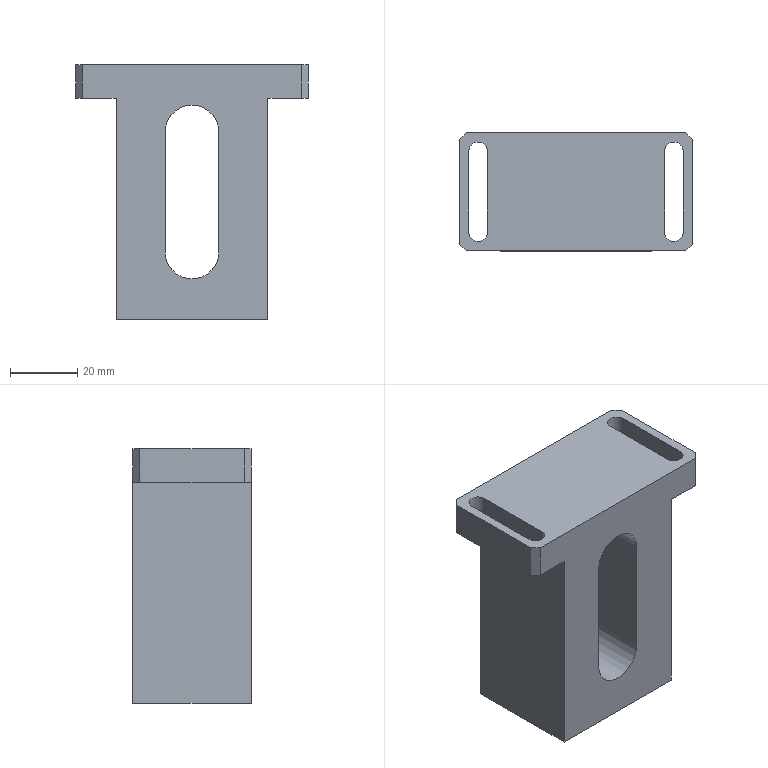Part | STEP file | 11-FG-S01411 | 1 solid | 43 faces | box 69 x 35 x 75.5 mm | volume 96843 mm3 | plane 20 | cylinder 15 | cone 8 | commonest cylinder face diameters 3.3 x8 5.5 x4 16 x3
STEP:
#1=CARTESIAN_POINT('',(23.5,-35.,63.5));
#2=VERTEX_POINT('',#1);
#3=CARTESIAN_POINT('',(31.5,-35.,55.5));
#4=VERTEX_POINT('',#3);
#5=CARTESIAN_POINT('',(23.5,-35.,55.5));
#6=DIRECTION('',(0.,1.,0.));
#7=DIRECTION('',(0.,0.,1.));
#8=AXIS2_PLACEMENT_3D('',#5,#6,#7);
#9=CIRCLE('',#8,8.);
#10=EDGE_CURVE('',#2,#4,#9,.T.);
#11=ORIENTED_EDGE('',*,*,#10,.F.);
#12=CARTESIAN_POINT('',(23.5,0.,63.5));
#13=VERTEX_POINT('',#12);
#14=CARTESIAN_POINT('',(23.5,-40.,63.5));
#15=DIRECTION('',(0.,1.,0.));
#16=VECTOR('',#15,1000.);
#17=LINE('',#14,#16);
#18=EDGE_CURVE('',#2,#13,#17,.T.);
#19=ORIENTED_EDGE('',*,*,#18,.T.);
#20=CARTESIAN_POINT('',(31.5,0.,55.5));
#21=VERTEX_POINT('',#20);
#22=CARTESIAN_POINT('',(23.5,0.,55.5));
#23=DIRECTION('',(0.,1.,0.));
#24=DIRECTION('',(0.,0.,1.));
#25=AXIS2_PLACEMENT_3D('',#22,#23,#24);
#26=CIRCLE('',#25,8.);
#27=EDGE_CURVE('',#13,#21,#26,.T.);
#28=ORIENTED_EDGE('',*,*,#27,.T.);
#29=CARTESIAN_POINT('',(31.5,-40.,55.5));
#30=DIRECTION('',(0.,1.,0.));
#31=VECTOR('',#30,1000.);
#32=LINE('',#29,#31);
#33=EDGE_CURVE('',#4,#21,#32,.T.);
#34=ORIENTED_EDGE('',*,*,#33,.F.);
#35=EDGE_LOOP('',(#11,#19,#28,#34));
#36=FACE_OUTER_BOUND('',#35,.T.);
#37=CARTESIAN_POINT('',(23.5,-40.,55.5));
#38=DIRECTION('',(0.,1.,0.));
#39=DIRECTION('',(0.,0.,1.));
#40=AXIS2_PLACEMENT_3D('',#37,#38,#39);
#41=CYLINDRICAL_SURFACE('',#40,8.);
#42=ADVANCED_FACE('',(#36),#41,.F.);
#43=CARTESIAN_POINT('',(44.15,-7.,10.1));
#44=VERTEX_POINT('',#43);
#45=CARTESIAN_POINT('',(40.85,-7.,10.1));
#46=VERTEX_POINT('',#45);
#47=CARTESIAN_POINT('',(42.5,-7.,10.1));
#48=DIRECTION('',(0.,0.,-1.));
#49=DIRECTION('',(-1.,0.,0.));
#50=AXIS2_PLACEMENT_3D('',#47,#48,#49);
#51=CIRCLE('',#50,1.65);
#52=EDGE_CURVE('',#44,#46,#51,.T.);
#53=ORIENTED_EDGE('',*,*,#52,.F.);
#54=CARTESIAN_POINT('',(44.15,-7.,0.));
#55=VERTEX_POINT('',#54);
#56=CARTESIAN_POINT('',(44.15,-7.,0.));
#57=DIRECTION('',(0.,0.,-1.));
#58=VECTOR('',#57,1000.);
#59=LINE('',#56,#58);
#60=EDGE_CURVE('',#44,#55,#59,.T.);
#61=ORIENTED_EDGE('',*,*,#60,.T.);
#62=CARTESIAN_POINT('',(40.85,-7.,0.));
#63=VERTEX_POINT('',#62);
#64=CARTESIAN_POINT('',(42.5,-7.,0.));
#65=DIRECTION('',(0.,0.,-1.));
#66=DIRECTION('',(-1.,0.,0.));
#67=AXIS2_PLACEMENT_3D('',#64,#65,#66);
#68=CIRCLE('',#67,1.65);
#69=EDGE_CURVE('',#55,#63,#68,.T.);
#70=ORIENTED_EDGE('',*,*,#69,.T.);
#71=CARTESIAN_POINT('',(40.85,-7.,0.));
#72=DIRECTION('',(0.,0.,-1.));
#73=VECTOR('',#72,1000.);
#74=LINE('',#71,#73);
#75=EDGE_CURVE('',#46,#63,#74,.T.);
#76=ORIENTED_EDGE('',*,*,#75,.F.);
#77=EDGE_LOOP('',(#53,#61,#70,#76));
#78=FACE_OUTER_BOUND('',#77,.T.);
#79=CARTESIAN_POINT('',(42.5,-7.,0.));
#80=DIRECTION('',(0.,0.,-1.));
#81=DIRECTION('',(-1.,0.,0.));
#82=AXIS2_PLACEMENT_3D('',#79,#80,#81);
#83=CYLINDRICAL_SURFACE('',#82,1.65);
#84=ADVANCED_FACE('',(#78),#83,.F.);
#85=CARTESIAN_POINT('',(42.5,-7.,11.091));
#86=VERTEX_POINT('',#85);
#87=CARTESIAN_POINT('',(40.85,-7.,10.1));
#88=DIRECTION('',(-0.8572,0.,-0.515));
#89=VECTOR('',#88,1000.);
#90=LINE('',#87,#89);
#91=EDGE_CURVE('',#86,#46,#90,.T.);
#92=ORIENTED_EDGE('',*,*,#91,.F.);
#93=CARTESIAN_POINT('',(44.15,-7.,10.1));
#94=DIRECTION('',(0.8572,0.,-0.515));
#95=VECTOR('',#94,1000.);
#96=LINE('',#93,#95);
#97=EDGE_CURVE('',#86,#44,#96,.T.);
#98=ORIENTED_EDGE('',*,*,#97,.T.);
#99=ORIENTED_EDGE('',*,*,#52,.T.);
#100=EDGE_LOOP('',(#92,#98,#99));
#101=FACE_OUTER_BOUND('',#100,.T.);
#102=CARTESIAN_POINT('',(42.5,-7.,10.1));
#103=DIRECTION('',(0.,0.,-1.));
#104=DIRECTION('',(-1.,0.,0.));
#105=AXIS2_PLACEMENT_3D('',#102,#103,#104);
#106=CONICAL_SURFACE('',#105,1.65,1.03);
#107=ADVANCED_FACE('',(#101),#106,.F.);
#108=CARTESIAN_POINT('',(44.15,-28.,10.1));
#109=VERTEX_POINT('',#108);
#110=CARTESIAN_POINT('',(40.85,-28.,10.1));
#111=VERTEX_POINT('',#110);
#112=CARTESIAN_POINT('',(42.5,-28.,10.1));
#113=DIRECTION('',(0.,0.,-1.));
#114=DIRECTION('',(-1.,0.,0.));
#115=AXIS2_PLACEMENT_3D('',#112,#113,#114);
#116=CIRCLE('',#115,1.65);
#117=EDGE_CURVE('',#109,#111,#116,.T.);
#118=ORIENTED_EDGE('',*,*,#117,.F.);
#119=CARTESIAN_POINT('',(44.15,-28.,0.));
#120=VERTEX_POINT('',#119);
#121=CARTESIAN_POINT('',(44.15,-28.,0.));
#122=DIRECTION('',(0.,0.,-1.));
#123=VECTOR('',#122,1000.);
#124=LINE('',#121,#123);
#125=EDGE_CURVE('',#109,#120,#124,.T.);
#126=ORIENTED_EDGE('',*,*,#125,.T.);
#127=CARTESIAN_POINT('',(40.85,-28.,0.));
#128=VERTEX_POINT('',#127);
#129=CARTESIAN_POINT('',(42.5,-28.,0.));
#130=DIRECTION('',(0.,0.,-1.));
#131=DIRECTION('',(-1.,0.,0.));
#132=AXIS2_PLACEMENT_3D('',#129,#130,#131);
#133=CIRCLE('',#132,1.65);
#134=EDGE_CURVE('',#120,#128,#133,.T.);
#135=ORIENTED_EDGE('',*,*,#134,.T.);
#136=CARTESIAN_POINT('',(40.85,-28.,0.));
#137=DIRECTION('',(0.,0.,-1.));
#138=VECTOR('',#137,1000.);
#139=LINE('',#136,#138);
#140=EDGE_CURVE('',#111,#128,#139,.T.);
#141=ORIENTED_EDGE('',*,*,#140,.F.);
#142=EDGE_LOOP('',(#118,#126,#135,#141));
#143=FACE_OUTER_BOUND('',#142,.T.);
#144=CARTESIAN_POINT('',(42.5,-28.,0.));
#145=DIRECTION('',(0.,0.,-1.));
#146=DIRECTION('',(-1.,0.,0.));
#147=AXIS2_PLACEMENT_3D('',#144,#145,#146);
#148=CYLINDRICAL_SURFACE('',#147,1.65);
#149=ADVANCED_FACE('',(#143),#148,.F.);
#150=CARTESIAN_POINT('',(42.5,-28.,11.091));
#151=VERTEX_POINT('',#150);
#152=CARTESIAN_POINT('',(40.85,-28.,10.1));
#153=DIRECTION('',(-0.8572,0.,-0.515));
#154=VECTOR('',#153,1000.);
#155=LINE('',#152,#154);
#156=EDGE_CURVE('',#151,#111,#155,.T.);
#157=ORIENTED_EDGE('',*,*,#156,.F.);
#158=CARTESIAN_POINT('',(44.15,-28.,10.1));
#159=DIRECTION('',(0.8572,0.,-0.515));
#160=VECTOR('',#159,1000.);
#161=LINE('',#158,#160);
#162=EDGE_CURVE('',#151,#109,#161,.T.);
#163=ORIENTED_EDGE('',*,*,#162,.T.);
#164=ORIENTED_EDGE('',*,*,#117,.T.);
#165=EDGE_LOOP('',(#157,#163,#164));
#166=FACE_OUTER_BOUND('',#165,.T.);
#167=CARTESIAN_POINT('',(42.5,-28.,10.1));
#168=DIRECTION('',(0.,0.,-1.));
#169=DIRECTION('',(-1.,0.,0.));
#170=AXIS2_PLACEMENT_3D('',#167,#168,#169);
#171=CONICAL_SURFACE('',#170,1.65,1.03);
#172=ADVANCED_FACE('',(#166),#171,.F.);
#173=CARTESIAN_POINT('',(6.15,-7.,10.1));
#174=VERTEX_POINT('',#173);
#175=CARTESIAN_POINT('',(2.85,-7.,10.1));
#176=VERTEX_POINT('',#175);
#177=CARTESIAN_POINT('',(4.5,-7.,10.1));
#178=DIRECTION('',(0.,0.,-1.));
#179=DIRECTION('',(-1.,0.,0.));
#180=AXIS2_PLACEMENT_3D('',#177,#178,#179);
#181=CIRCLE('',#180,1.65);
#182=EDGE_CURVE('',#174,#176,#181,.T.);
#183=ORIENTED_EDGE('',*,*,#182,.F.);
#184=CARTESIAN_POINT('',(6.15,-7.,0.));
#185=VERTEX_POINT('',#184);
#186=CARTESIAN_POINT('',(6.15,-7.,0.));
#187=DIRECTION('',(0.,0.,-1.));
#188=VECTOR('',#187,1000.);
#189=LINE('',#186,#188);
#190=EDGE_CURVE('',#174,#185,#189,.T.);
#191=ORIENTED_EDGE('',*,*,#190,.T.);
#192=CARTESIAN_POINT('',(2.85,-7.,0.));
#193=VERTEX_POINT('',#192);
#194=CARTESIAN_POINT('',(4.5,-7.,0.));
#195=DIRECTION('',(0.,0.,-1.));
#196=DIRECTION('',(-1.,0.,0.));
#197=AXIS2_PLACEMENT_3D('',#194,#195,#196);
#198=CIRCLE('',#197,1.65);
#199=EDGE_CURVE('',#185,#193,#198,.T.);
#200=ORIENTED_EDGE('',*,*,#199,.T.);
#201=CARTESIAN_POINT('',(2.85,-7.,0.));
#202=DIRECTION('',(0.,0.,-1.));
#203=VECTOR('',#202,1000.);
#204=LINE('',#201,#203);
#205=EDGE_CURVE('',#176,#193,#204,.T.);
#206=ORIENTED_EDGE('',*,*,#205,.F.);
#207=EDGE_LOOP('',(#183,#191,#200,#206));
#208=FACE_OUTER_BOUND('',#207,.T.);
#209=CARTESIAN_POINT('',(4.5,-7.,0.));
#210=DIRECTION('',(0.,0.,-1.));
#211=DIRECTION('',(-1.,0.,0.));
#212=AXIS2_PLACEMENT_3D('',#209,#210,#211);
#213=CYLINDRICAL_SURFACE('',#212,1.65);
#214=ADVANCED_FACE('',(#208),#213,.F.);
#215=CARTESIAN_POINT('',(4.5,-7.,11.091));
#216=VERTEX_POINT('',#215);
#217=CARTESIAN_POINT('',(2.85,-7.,10.1));
#218=DIRECTION('',(-0.8572,0.,-0.515));
#219=VECTOR('',#218,1000.);
#220=LINE('',#217,#219);
#221=EDGE_CURVE('',#216,#176,#220,.T.);
#222=ORIENTED_EDGE('',*,*,#221,.F.);
#223=CARTESIAN_POINT('',(6.15,-7.,10.1));
#224=DIRECTION('',(0.8572,0.,-0.515));
#225=VECTOR('',#224,1000.);
#226=LINE('',#223,#225);
#227=EDGE_CURVE('',#216,#174,#226,.T.);
#228=ORIENTED_EDGE('',*,*,#227,.T.);
#229=ORIENTED_EDGE('',*,*,#182,.T.);
#230=EDGE_LOOP('',(#222,#228,#229));
#231=FACE_OUTER_BOUND('',#230,.T.);
#232=CARTESIAN_POINT('',(4.5,-7.,10.1));
#233=DIRECTION('',(0.,0.,-1.));
#234=DIRECTION('',(-1.,0.,0.));
#235=AXIS2_PLACEMENT_3D('',#232,#233,#234);
#236=CONICAL_SURFACE('',#235,1.65,1.03);
#237=ADVANCED_FACE('',(#231),#236,.F.);
#238=CARTESIAN_POINT('',(6.15,-28.,10.1));
#239=VERTEX_POINT('',#238);
#240=CARTESIAN_POINT('',(2.85,-28.,10.1));
#241=VERTEX_POINT('',#240);
#242=CARTESIAN_POINT('',(4.5,-28.,10.1));
#243=DIRECTION('',(0.,0.,-1.));
#244=DIRECTION('',(-1.,0.,0.));
#245=AXIS2_PLACEMENT_3D('',#242,#243,#244);
#246=CIRCLE('',#245,1.65);
#247=EDGE_CURVE('',#239,#241,#246,.T.);
#248=ORIENTED_EDGE('',*,*,#247,.F.);
#249=CARTESIAN_POINT('',(6.15,-28.,0.));
#250=VERTEX_POINT('',#249);
#251=CARTESIAN_POINT('',(6.15,-28.,0.));
#252=DIRECTION('',(0.,0.,-1.));
#253=VECTOR('',#252,1000.);
#254=LINE('',#251,#253);
#255=EDGE_CURVE('',#239,#250,#254,.T.);
#256=ORIENTED_EDGE('',*,*,#255,.T.);
#257=CARTESIAN_POINT('',(2.85,-28.,0.));
#258=VERTEX_POINT('',#257);
#259=CARTESIAN_POINT('',(4.5,-28.,0.));
#260=DIRECTION('',(0.,0.,-1.));
#261=DIRECTION('',(-1.,0.,0.));
#262=AXIS2_PLACEMENT_3D('',#259,#260,#261);
#263=CIRCLE('',#262,1.65);
#264=EDGE_CURVE('',#250,#258,#263,.T.);
#265=ORIENTED_EDGE('',*,*,#264,.T.);
#266=CARTESIAN_POINT('',(2.85,-28.,0.));
#267=DIRECTION('',(0.,0.,-1.));
#268=VECTOR('',#267,1000.);
#269=LINE('',#266,#268);
#270=EDGE_CURVE('',#241,#258,#269,.T.);
#271=ORIENTED_EDGE('',*,*,#270,.F.);
#272=EDGE_LOOP('',(#248,#256,#265,#271));
#273=FACE_OUTER_BOUND('',#272,.T.);
#274=CARTESIAN_POINT('',(4.5,-28.,0.));
#275=DIRECTION('',(0.,0.,-1.));
#276=DIRECTION('',(-1.,0.,0.));
#277=AXIS2_PLACEMENT_3D('',#274,#275,#276);
#278=CYLINDRICAL_SURFACE('',#277,1.65);
#279=ADVANCED_FACE('',(#273),#278,.F.);
#280=CARTESIAN_POINT('',(4.5,-28.,11.091));
#281=VERTEX_POINT('',#280);
#282=CARTESIAN_POINT('',(2.85,-28.,10.1));
#283=DIRECTION('',(-0.8572,0.,-0.515));
#284=VECTOR('',#283,1000.);
#285=LINE('',#282,#284);
#286=EDGE_CURVE('',#281,#241,#285,.T.);
#287=ORIENTED_EDGE('',*,*,#286,.F.);
#288=CARTESIAN_POINT('',(6.15,-28.,10.1));
#289=DIRECTION('',(0.8572,0.,-0.515));
#290=VECTOR('',#289,1000.);
#291=LINE('',#288,#290);
#292=EDGE_CURVE('',#281,#239,#291,.T.);
#293=ORIENTED_EDGE('',*,*,#292,.T.);
#294=ORIENTED_EDGE('',*,*,#247,.T.);
#295=EDGE_LOOP('',(#287,#293,#294));
#296=FACE_OUTER_BOUND('',#295,.T.);
#297=CARTESIAN_POINT('',(4.5,-28.,10.1));
#298=DIRECTION('',(0.,0.,-1.));
#299=DIRECTION('',(-1.,0.,0.));
#300=AXIS2_PLACEMENT_3D('',#297,#298,#299);
#301=CONICAL_SURFACE('',#300,1.65,1.03);
#302=ADVANCED_FACE('',(#296),#301,.F.);
#303=CARTESIAN_POINT('',(31.5,-35.,20.));
#304=VERTEX_POINT('',#303);
#305=CARTESIAN_POINT('',(31.5,-35.,75.5));
#306=DIRECTION('',(0.,0.,-1.));
#307=VECTOR('',#306,1000.);
#308=LINE('',#305,#307);
#309=EDGE_CURVE('',#4,#304,#308,.T.);
#310=ORIENTED_EDGE('',*,*,#309,.T.);
#311=CARTESIAN_POINT('',(15.5,-35.,20.));
#312=VERTEX_POINT('',#311);
#313=CARTESIAN_POINT('',(23.5,-35.,20.));
#314=DIRECTION('',(0.,1.,0.));
#315=DIRECTION('',(0.,0.,1.));
#316=AXIS2_PLACEMENT_3D('',#313,#314,#315);
#317=CIRCLE('',#316,8.);
#318=EDGE_CURVE('',#304,#312,#317,.T.);
#319=ORIENTED_EDGE('',*,*,#318,.T.);
#320=CARTESIAN_POINT('',(15.5,-35.,55.5));
#321=VERTEX_POINT('',#320);
#322=CARTESIAN_POINT('',(15.5,-35.,75.5));
#323=DIRECTION('',(0.,0.,1.));
#324=VECTOR('',#323,1000.);
#325=LINE('',#322,#324);
#326=EDGE_CURVE('',#312,#321,#325,.T.);
#327=ORIENTED_EDGE('',*,*,#326,.T.);
#328=CARTESIAN_POINT('',(23.5,-35.,55.5));
#329=DIRECTION('',(0.,1.,0.));
#330=DIRECTION('',(0.,0.,1.));
#331=AXIS2_PLACEMENT_3D('',#328,#329,#330);
#332=CIRCLE('',#331,8.);
#333=EDGE_CURVE('',#321,#2,#332,.T.);
#334=ORIENTED_EDGE('',*,*,#333,.T.);
#335=ORIENTED_EDGE('',*,*,#10,.T.);
#336=EDGE_LOOP('',(#310,#319,#327,#334,#335));
#337=FACE_BOUND('',#336,.T.);
#338=CARTESIAN_POINT('',(-9.,-35.,75.5));
#339=VERTEX_POINT('',#338);
#340=CARTESIAN_POINT('',(56.,-35.,75.5));
#341=VERTEX_POINT('',#340);
#342=CARTESIAN_POINT('',(0.,-35.,75.5));
#343=DIRECTION('',(1.,0.,0.));
#344=VECTOR('',#343,1000.);
#345=LINE('',#342,#344);
#346=EDGE_CURVE('',#339,#341,#345,.T.);
#347=ORIENTED_EDGE('',*,*,#346,.F.);
#348=CARTESIAN_POINT('',(-9.,-35.,65.5));
#349=VERTEX_POINT('',#348);
#350=CARTESIAN_POINT('',(-9.,-35.,65.5));
#351=DIRECTION('',(0.,0.,-1.));
#352=VECTOR('',#351,1000.);
#353=LINE('',#350,#352);
#354=EDGE_CURVE('',#339,#349,#353,.T.);
#355=ORIENTED_EDGE('',*,*,#354,.T.);
#356=CARTESIAN_POINT('',(1.,-35.,65.5));
#357=VERTEX_POINT('',#356);
#358=CARTESIAN_POINT('',(1.,-35.,65.5));
#359=DIRECTION('',(1.,0.,0.));
#360=VECTOR('',#359,1000.);
#361=LINE('',#358,#360);
#362=EDGE_CURVE('',#349,#357,#361,.T.);
#363=ORIENTED_EDGE('',*,*,#362,.T.);
#364=CARTESIAN_POINT('',(1.,-35.,0.));
#365=VERTEX_POINT('',#364);
#366=CARTESIAN_POINT('',(1.,-35.,75.5));
#367=DIRECTION('',(0.,0.,-1.));
#368=VECTOR('',#367,1000.);
#369=LINE('',#366,#368);
#370=EDGE_CURVE('',#357,#365,#369,.T.);
#371=ORIENTED_EDGE('',*,*,#370,.T.);
#372=CARTESIAN_POINT('',(46.,-35.,0.));
#373=VERTEX_POINT('',#372);
#374=CARTESIAN_POINT('',(0.,-35.,0.));
#375=DIRECTION('',(1.,0.,0.));
#376=VECTOR('',#375,1000.);
#377=LINE('',#374,#376);
#378=EDGE_CURVE('',#365,#373,#377,.T.);
#379=ORIENTED_EDGE('',*,*,#378,.T.);
#380=CARTESIAN_POINT('',(46.,-35.,65.5));
#381=VERTEX_POINT('',#380);
#382=CARTESIAN_POINT('',(46.,-35.,75.5));
#383=DIRECTION('',(0.,0.,-1.));
#384=VECTOR('',#383,1000.);
#385=LINE('',#382,#384);
#386=EDGE_CURVE('',#381,#373,#385,.T.);
#387=ORIENTED_EDGE('',*,*,#386,.F.);
#388=CARTESIAN_POINT('',(56.,-35.,65.5));
#389=VERTEX_POINT('',#388);
#390=CARTESIAN_POINT('',(46.,-35.,65.5));
#391=DIRECTION('',(1.,0.,0.));
#392=VECTOR('',#391,1000.);
#393=LINE('',#390,#392);
#394=EDGE_CURVE('',#381,#389,#393,.T.);
#395=ORIENTED_EDGE('',*,*,#394,.T.);
#396=CARTESIAN_POINT('',(56.,-35.,75.5));
#397=DIRECTION('',(0.,0.,1.));
#398=VECTOR('',#397,1000.);
#399=LINE('',#396,#398);
#400=EDGE_CURVE('',#389,#341,#399,.T.);
#401=ORIENTED_EDGE('',*,*,#400,.T.);
#402=EDGE_LOOP('',(#347,#355,#363,#371,#379,#387,#395,#401));
#403=FACE_OUTER_BOUND('',#402,.T.);
#404=CARTESIAN_POINT('',(0.,-35.,75.5));
#405=DIRECTION('',(0.,1.,0.));
#406=DIRECTION('',(0.,0.,1.));
#407=AXIS2_PLACEMENT_3D('',#404,#405,#406);
#408=PLANE('',#407);
#409=ADVANCED_FACE('',(#337,#403),#408,.F.);
#410=CARTESIAN_POINT('',(46.,0.,65.5));
#411=VERTEX_POINT('',#410);
#412=CARTESIAN_POINT('',(46.,0.,0.));
#413=VERTEX_POINT('',#412);
#414=CARTESIAN_POINT('',(46.,0.,75.5));
#415=DIRECTION('',(0.,0.,-1.));
#416=VECTOR('',#415,1000.);
#417=LINE('',#414,#416);
#418=EDGE_CURVE('',#411,#413,#417,.T.);
#419=ORIENTED_EDGE('',*,*,#418,.F.);
#420=CARTESIAN_POINT('',(46.,0.,65.5));
#421=DIRECTION('',(0.,-1.,0.));
#422=VECTOR('',#421,1000.);
#423=LINE('',#420,#422);
#424=EDGE_CURVE('',#411,#381,#423,.T.);
#425=ORIENTED_EDGE('',*,*,#424,.T.);
#426=ORIENTED_EDGE('',*,*,#386,.T.);
#427=CARTESIAN_POINT('',(46.,0.,0.));
#428=DIRECTION('',(0.,1.,0.));
#429=VECTOR('',#428,1000.);
#430=LINE('',#427,#429);
#431=EDGE_CURVE('',#373,#413,#430,.T.);
#432=ORIENTED_EDGE('',*,*,#431,.T.);
#433=EDGE_LOOP('',(#419,#425,#426,#432));
#434=FACE_OUTER_BOUND('',#433,.T.);
#435=CARTESIAN_POINT('',(46.,0.,75.5));
#436=DIRECTION('',(-1.,0.,0.));
#437=DIRECTION('',(0.,0.,1.));
#438=AXIS2_PLACEMENT_3D('',#435,#436,#437);
#439=PLANE('',#438);
#440=ADVANCED_FACE('',(#434),#439,.F.);
#441=CARTESIAN_POINT('',(15.5,0.,20.));
#442=VERTEX_POINT('',#441);
#443=CARTESIAN_POINT('',(15.5,0.,55.5));
#444=VERTEX_POINT('',#443);
#445=CARTESIAN_POINT('',(15.5,0.,20.));
#446=DIRECTION('',(0.,0.,1.));
#447=VECTOR('',#446,1000.);
#448=LINE('',#445,#447);
#449=EDGE_CURVE('',#442,#444,#448,.T.);
#450=ORIENTED_EDGE('',*,*,#449,.F.);
#451=CARTESIAN_POINT('',(31.5,0.,20.));
#452=VERTEX_POINT('',#451);
#453=CARTESIAN_POINT('',(23.5,0.,20.));
#454=DIRECTION('',(0.,1.,0.));
#455=DIRECTION('',(0.,0.,1.));
#456=AXIS2_PLACEMENT_3D('',#453,#454,#455);
#457=CIRCLE('',#456,8.);
#458=EDGE_CURVE('',#452,#442,#457,.T.);
#459=ORIENTED_EDGE('',*,*,#458,.F.);
#460=CARTESIAN_POINT('',(31.5,0.,20.));
#461=DIRECTION('',(0.,0.,-1.));
#462=VECTOR('',#461,1000.);
#463=LINE('',#460,#462);
#464=EDGE_CURVE('',#21,#452,#463,.T.);
#465=ORIENTED_EDGE('',*,*,#464,.F.);
#466=ORIENTED_EDGE('',*,*,#27,.F.);
#467=CARTESIAN_POINT('',(23.5,0.,55.5));
#468=DIRECTION('',(0.,1.,0.));
#469=DIRECTION('',(0.,0.,1.));
#470=AXIS2_PLACEMENT_3D('',#467,#468,#469);
#471=CIRCLE('',#470,8.);
#472=EDGE_CURVE('',#444,#13,#471,.T.);
#473=ORIENTED_EDGE('',*,*,#472,.F.);
#474=EDGE_LOOP('',(#450,#459,#465,#466,#473));
#475=FACE_BOUND('',#474,.T.);
#476=CARTESIAN_POINT('',(1.,0.,65.5));
#477=VERTEX_POINT('',#476);
#478=CARTESIAN_POINT('',(-9.,0.,65.5));
#479=VERTEX_POINT('',#478);
#480=CARTESIAN_POINT('',(1.,0.,65.5));
#481=DIRECTION('',(-1.,0.,0.));
#482=VECTOR('',#481,1000.);
#483=LINE('',#480,#482);
#484=EDGE_CURVE('',#477,#479,#483,.T.);
#485=ORIENTED_EDGE('',*,*,#484,.T.);
#486=CARTESIAN_POINT('',(-9.,0.,75.5));
#487=VERTEX_POINT('',#486);
#488=CARTESIAN_POINT('',(-9.,0.,75.5));
#489=DIRECTION('',(0.,0.,1.));
#490=VECTOR('',#489,1000.);
#491=LINE('',#488,#490);
#492=EDGE_CURVE('',#479,#487,#491,.T.);
#493=ORIENTED_EDGE('',*,*,#492,.T.);
#494=CARTESIAN_POINT('',(56.,0.,75.5));
#495=VERTEX_POINT('',#494);
#496=CARTESIAN_POINT('',(0.,0.,75.5));
#497=DIRECTION('',(-1.,0.,0.));
#498=VECTOR('',#497,1000.);
#499=LINE('',#496,#498);
#500=EDGE_CURVE('',#495,#487,#499,.T.);
#501=ORIENTED_EDGE('',*,*,#500,.F.);
#502=CARTESIAN_POINT('',(56.,0.,65.5));
#503=VERTEX_POINT('',#502);
#504=CARTESIAN_POINT('',(56.,0.,65.5));
#505=DIRECTION('',(0.,0.,-1.));
#506=VECTOR('',#505,1000.);
#507=LINE('',#504,#506);
#508=EDGE_CURVE('',#495,#503,#507,.T.);
#509=ORIENTED_EDGE('',*,*,#508,.T.);
#510=CARTESIAN_POINT('',(46.,0.,65.5));
#511=DIRECTION('',(-1.,0.,0.));
#512=VECTOR('',#511,1000.);
#513=LINE('',#510,#512);
#514=EDGE_CURVE('',#503,#411,#513,.T.);
#515=ORIENTED_EDGE('',*,*,#514,.T.);
#516=ORIENTED_EDGE('',*,*,#418,.T.);
#517=CARTESIAN_POINT('',(1.,0.,0.));
#518=VERTEX_POINT('',#517);
#519=CARTESIAN_POINT('',(0.,0.,0.));
#520=DIRECTION('',(-1.,0.,0.));
#521=VECTOR('',#520,1000.);
#522=LINE('',#519,#521);
#523=EDGE_CURVE('',#413,#518,#522,.T.);
#524=ORIENTED_EDGE('',*,*,#523,.T.);
#525=CARTESIAN_POINT('',(1.,0.,0.));
#526=DIRECTION('',(0.,0.,-1.));
#527=VECTOR('',#526,1000.);
#528=LINE('',#525,#527);
#529=EDGE_CURVE('',#477,#518,#528,.T.);
#530=ORIENTED_EDGE('',*,*,#529,.F.);
#531=EDGE_LOOP('',(#485,#493,#501,#509,#515,#516,#524,#530));
#532=FACE_OUTER_BOUND('',#531,.T.);
#533=CARTESIAN_POINT('',(0.,0.,75.5));
#534=DIRECTION('',(0.,-1.,0.));
#535=DIRECTION('',(0.,0.,-1.));
#536=AXIS2_PLACEMENT_3D('',#533,#534,#535);
#537=PLANE('',#536);
#538=ADVANCED_FACE('',(#475,#532),#537,.F.);
#539=CARTESIAN_POINT('',(-8.25,-5.5,75.5));
#540=VERTEX_POINT('',#539);
#541=CARTESIAN_POINT('',(-2.75,-5.5,75.5));
#542=VERTEX_POINT('',#541);
#543=CARTESIAN_POINT('',(-5.5,-5.5,75.5));
#544=DIRECTION('',(0.,0.,-1.));
#545=DIRECTION('',(-1.,0.,0.));
#546=AXIS2_PLACEMENT_3D('',#543,#544,#545);
#547=CIRCLE('',#546,2.75);
#548=EDGE_CURVE('',#540,#542,#547,.T.);
#549=ORIENTED_EDGE('',*,*,#548,.T.);
#550=CARTESIAN_POINT('',(-2.75,-29.5,75.5));
#551=VERTEX_POINT('',#550);
#552=CARTESIAN_POINT('',(-2.75,-5.5,75.5));
#553=DIRECTION('',(0.,-1.,0.));
#554=VECTOR('',#553,1000.);
#555=LINE('',#552,#554);
#556=EDGE_CURVE('',#542,#551,#555,.T.);
#557=ORIENTED_EDGE('',*,*,#556,.T.);
#558=CARTESIAN_POINT('',(-8.25,-29.5,75.5));
#559=VERTEX_POINT('',#558);
#560=CARTESIAN_POINT('',(-5.5,-29.5,75.5));
#561=DIRECTION('',(0.,0.,-1.));
#562=DIRECTION('',(-1.,0.,0.));
#563=AXIS2_PLACEMENT_3D('',#560,#561,#562);
#564=CIRCLE('',#563,2.75);
#565=EDGE_CURVE('',#551,#559,#564,.T.);
#566=ORIENTED_EDGE('',*,*,#565,.T.);
#567=CARTESIAN_POINT('',(-8.25,-5.5,75.5));
#568=DIRECTION('',(0.,1.,0.));
#569=VECTOR('',#568,1000.);
#570=LINE('',#567,#569);
#571=EDGE_CURVE('',#559,#540,#570,.T.);
#572=ORIENTED_EDGE('',*,*,#571,.T.);
#573=EDGE_LOOP('',(#549,#557,#566,#572));
#574=FACE_BOUND('',#573,.T.);
#575=CARTESIAN_POINT('',(49.75,-5.5,75.5));
#576=VERTEX_POINT('',#575);
#577=CARTESIAN_POINT('',(55.25,-5.5,75.5));
#578=VERTEX_POINT('',#577);
#579=CARTESIAN_POINT('',(52.5,-5.5,75.5));
#580=DIRECTION('',(0.,0.,-1.));
#581=DIRECTION('',(-1.,0.,0.));
#582=AXIS2_PLACEMENT_3D('',#579,#580,#581);
#583=CIRCLE('',#582,2.75);
#584=EDGE_CURVE('',#576,#578,#583,.T.);
#585=ORIENTED_EDGE('',*,*,#584,.T.);
#586=CARTESIAN_POINT('',(55.25,-29.5,75.5));
#587=VERTEX_POINT('',#586);
#588=CARTESIAN_POINT('',(55.25,-5.5,75.5));
#589=DIRECTION('',(0.,-1.,0.));
#590=VECTOR('',#589,1000.);
#591=LINE('',#588,#590);
#592=EDGE_CURVE('',#578,#587,#591,.T.);
#593=ORIENTED_EDGE('',*,*,#592,.T.);
#594=CARTESIAN_POINT('',(49.75,-29.5,75.5));
#595=VERTEX_POINT('',#594);
#596=CARTESIAN_POINT('',(52.5,-29.5,75.5));
#597=DIRECTION('',(0.,0.,-1.));
#598=DIRECTION('',(-1.,0.,0.));
#599=AXIS2_PLACEMENT_3D('',#596,#597,#598);
#600=CIRCLE('',#599,2.75);
#601=EDGE_CURVE('',#587,#595,#600,.T.);
#602=ORIENTED_EDGE('',*,*,#601,.T.);
#603=CARTESIAN_POINT('',(49.75,-5.5,75.5));
#604=DIRECTION('',(0.,1.,0.));
#605=VECTOR('',#604,1000.);
#606=LINE('',#603,#605);
#607=EDGE_CURVE('',#595,#576,#606,.T.);
#608=ORIENTED_EDGE('',*,*,#607,.T.);
#609=EDGE_LOOP('',(#585,#593,#602,#608));
#610=FACE_BOUND('',#609,.T.);
#611=CARTESIAN_POINT('',(-11.,-2.,75.5));
#612=VERTEX_POINT('',#611);
#613=CARTESIAN_POINT('',(-11.,-33.,75.5));
#614=VERTEX_POINT('',#613);
#615=CARTESIAN_POINT('',(-11.,0.,75.5));
#616=DIRECTION('',(0.,-1.,0.));
#617=VECTOR('',#616,1000.);
#618=LINE('',#615,#617);
#619=EDGE_CURVE('',#612,#614,#618,.T.);
#620=ORIENTED_EDGE('',*,*,#619,.T.);
#621=CARTESIAN_POINT('',(-22.,-22.,75.5));
#622=DIRECTION('',(0.7071,-0.7071,0.));
#623=VECTOR('',#622,1000.);
#624=LINE('',#621,#623);
#625=EDGE_CURVE('',#614,#339,#624,.T.);
#626=ORIENTED_EDGE('',*,*,#625,.T.);
#627=ORIENTED_EDGE('',*,*,#346,.T.);
#628=CARTESIAN_POINT('',(58.,-33.,75.5));
#629=VERTEX_POINT('',#628);
#630=CARTESIAN_POINT('',(45.5,-45.5,75.5));
#631=DIRECTION('',(0.7071,0.7071,0.));
#632=VECTOR('',#631,1000.);
#633=LINE('',#630,#632);
#634=EDGE_CURVE('',#341,#629,#633,.T.);
#635=ORIENTED_EDGE('',*,*,#634,.T.);
#636=CARTESIAN_POINT('',(58.,-2.,75.5));
#637=VERTEX_POINT('',#636);
#638=CARTESIAN_POINT('',(58.,0.,75.5));
#639=DIRECTION('',(0.,1.,0.));
#640=VECTOR('',#639,1000.);
#641=LINE('',#638,#640);
#642=EDGE_CURVE('',#629,#637,#641,.T.);
#643=ORIENTED_EDGE('',*,*,#642,.T.);
#644=CARTESIAN_POINT('',(28.,28.,75.5));
#645=DIRECTION('',(-0.7071,0.7071,0.));
#646=VECTOR('',#645,1000.);
#647=LINE('',#644,#646);
#648=EDGE_CURVE('',#637,#495,#647,.T.);
#649=ORIENTED_EDGE('',*,*,#648,.T.);
#650=ORIENTED_EDGE('',*,*,#500,.T.);
#651=CARTESIAN_POINT('',(-4.5,4.5,75.5));
#652=DIRECTION('',(-0.7071,-0.7071,0.));
#653=VECTOR('',#652,1000.);
#654=LINE('',#651,#653);
#655=EDGE_CURVE('',#487,#612,#654,.T.);
#656=ORIENTED_EDGE('',*,*,#655,.T.);
#657=EDGE_LOOP('',(#620,#626,#627,#635,#643,#649,#650,#656));
#658=FACE_OUTER_BOUND('',#657,.T.);
#659=CARTESIAN_POINT('',(0.,0.,75.5));
#660=DIRECTION('',(0.,0.,1.));
#661=DIRECTION('',(1.,0.,0.));
#662=AXIS2_PLACEMENT_3D('',#659,#660,#661);
#663=PLANE('',#662);
#664=ADVANCED_FACE('',(#574,#610,#658),#663,.T.);
#665=CARTESIAN_POINT('',(42.5,-7.,0.));
#666=DIRECTION('',(0.,0.,-1.));
#667=DIRECTION('',(-1.,0.,0.));
#668=AXIS2_PLACEMENT_3D('',#665,#666,#667);
#669=CIRCLE('',#668,1.65);
#670=EDGE_CURVE('',#63,#55,#669,.T.);
#671=ORIENTED_EDGE('',*,*,#670,.F.);
#672=ORIENTED_EDGE('',*,*,#69,.F.);
#673=EDGE_LOOP('',(#671,#672));
#674=FACE_BOUND('',#673,.T.);
#675=CARTESIAN_POINT('',(42.5,-28.,0.));
#676=DIRECTION('',(0.,0.,-1.));
#677=DIRECTION('',(-1.,0.,0.));
#678=AXIS2_PLACEMENT_3D('',#675,#676,#677);
#679=CIRCLE('',#678,1.65);
#680=EDGE_CURVE('',#128,#120,#679,.T.);
#681=ORIENTED_EDGE('',*,*,#680,.F.);
#682=ORIENTED_EDGE('',*,*,#134,.F.);
#683=EDGE_LOOP('',(#681,#682));
#684=FACE_BOUND('',#683,.T.);
#685=CARTESIAN_POINT('',(4.5,-7.,0.));
#686=DIRECTION('',(0.,0.,-1.));
#687=DIRECTION('',(-1.,0.,0.));
#688=AXIS2_PLACEMENT_3D('',#685,#686,#687);
#689=CIRCLE('',#688,1.65);
#690=EDGE_CURVE('',#193,#185,#689,.T.);
#691=ORIENTED_EDGE('',*,*,#690,.F.);
#692=ORIENTED_EDGE('',*,*,#199,.F.);
#693=EDGE_LOOP('',(#691,#692));
#694=FACE_BOUND('',#693,.T.);
#695=CARTESIAN_POINT('',(4.5,-28.,0.));
#696=DIRECTION('',(0.,0.,-1.));
#697=DIRECTION('',(-1.,0.,0.));
#698=AXIS2_PLACEMENT_3D('',#695,#696,#697);
#699=CIRCLE('',#698,1.65);
#700=EDGE_CURVE('',#258,#250,#699,.T.);
#701=ORIENTED_EDGE('',*,*,#700,.F.);
#702=ORIENTED_EDGE('',*,*,#264,.F.);
#703=EDGE_LOOP('',(#701,#702));
#704=FACE_BOUND('',#703,.T.);
#705=ORIENTED_EDGE('',*,*,#378,.F.);
#706=CARTESIAN_POINT('',(1.,0.,0.));
#707=DIRECTION('',(0.,1.,0.));
#708=VECTOR('',#707,1000.);
#709=LINE('',#706,#708);
#710=EDGE_CURVE('',#365,#518,#709,.T.);
#711=ORIENTED_EDGE('',*,*,#710,.T.);
#712=ORIENTED_EDGE('',*,*,#523,.F.);
#713=ORIENTED_EDGE('',*,*,#431,.F.);
#714=EDGE_LOOP('',(#705,#711,#712,#713));
#715=FACE_OUTER_BOUND('',#714,.T.);
#716=CARTESIAN_POINT('',(0.,0.,0.));
#717=DIRECTION('',(0.,0.,1.));
#718=DIRECTION('',(1.,0.,0.));
#719=AXIS2_PLACEMENT_3D('',#716,#717,#718);
#720=PLANE('',#719);
#721=ADVANCED_FACE('',(#674,#684,#694,#704,#715),#720,.F.);
#722=ORIENTED_EDGE('',*,*,#370,.F.);
#723=CARTESIAN_POINT('',(1.,0.,65.5));
#724=DIRECTION('',(0.,1.,0.));
#725=VECTOR('',#724,1000.);
#726=LINE('',#723,#725);
#727=EDGE_CURVE('',#357,#477,#726,.T.);
#728=ORIENTED_EDGE('',*,*,#727,.T.);
#729=ORIENTED_EDGE('',*,*,#529,.T.);
#730=ORIENTED_EDGE('',*,*,#710,.F.);
#731=EDGE_LOOP('',(#722,#728,#729,#730));
#732=FACE_OUTER_BOUND('',#731,.T.);
#733=CARTESIAN_POINT('',(1.,-42.,0.));
#734=DIRECTION('',(1.,0.,0.));
#735=DIRECTION('',(0.,0.,-1.));
#736=AXIS2_PLACEMENT_3D('',#733,#734,#735);
#737=PLANE('',#736);
#738=ADVANCED_FACE('',(#732),#737,.F.);
#739=CARTESIAN_POINT('',(-11.,-2.,65.5));
#740=VERTEX_POINT('',#739);
#741=CARTESIAN_POINT('',(-11.,-33.,65.5));
#742=VERTEX_POINT('',#741);
#743=CARTESIAN_POINT('',(-11.,0.,65.5));
#744=DIRECTION('',(0.,-1.,0.));
#745=VECTOR('',#744,1000.);
#746=LINE('',#743,#745);
#747=EDGE_CURVE('',#740,#742,#746,.T.);
#748=ORIENTED_EDGE('',*,*,#747,.T.);
#749=CARTESIAN_POINT('',(-11.,-33.,75.5));
#750=DIRECTION('',(0.,0.,1.));
#751=VECTOR('',#750,1000.);
#752=LINE('',#749,#751);
#753=EDGE_CURVE('',#742,#614,#752,.T.);
#754=ORIENTED_EDGE('',*,*,#753,.T.);
#755=ORIENTED_EDGE('',*,*,#619,.F.);
#756=CARTESIAN_POINT('',(-11.,-2.,65.5));
#757=DIRECTION('',(0.,0.,-1.));
#758=VECTOR('',#757,1000.);
#759=LINE('',#756,#758);
#760=EDGE_CURVE('',#612,#740,#759,.T.);
#761=ORIENTED_EDGE('',*,*,#760,.T.);
#762=EDGE_LOOP('',(#748,#754,#755,#761));
#763=FACE_OUTER_BOUND('',#762,.T.);
#764=CARTESIAN_POINT('',(-11.,0.,65.5));
#765=DIRECTION('',(-1.,0.,0.));
#766=DIRECTION('',(0.,-1.,0.));
#767=AXIS2_PLACEMENT_3D('',#764,#765,#766);
#768=PLANE('',#767);
#769=ADVANCED_FACE('',(#763),#768,.T.);
#770=CARTESIAN_POINT('',(-8.25,-5.5,65.5));
#771=VERTEX_POINT('',#770);
#772=CARTESIAN_POINT('',(-2.75,-5.5,65.5));
#773=VERTEX_POINT('',#772);
#774=CARTESIAN_POINT('',(-5.5,-5.5,65.5));
#775=DIRECTION('',(0.,0.,-1.));
#776=DIRECTION('',(-1.,0.,0.));
#777=AXIS2_PLACEMENT_3D('',#774,#775,#776);
#778=CIRCLE('',#777,2.75);
#779=EDGE_CURVE('',#771,#773,#778,.T.);
#780=ORIENTED_EDGE('',*,*,#779,.F.);
#781=CARTESIAN_POINT('',(-8.25,-29.5,65.5));
#782=VERTEX_POINT('',#781);
#783=CARTESIAN_POINT('',(-8.25,-5.5,65.5));
#784=DIRECTION('',(0.,1.,0.));
#785=VECTOR('',#784,1000.);
#786=LINE('',#783,#785);
#787=EDGE_CURVE('',#782,#771,#786,.T.);
#788=ORIENTED_EDGE('',*,*,#787,.F.);
#789=CARTESIAN_POINT('',(-2.75,-29.5,65.5));
#790=VERTEX_POINT('',#789);
#791=CARTESIAN_POINT('',(-5.5,-29.5,65.5));
#792=DIRECTION('',(0.,0.,-1.));
#793=DIRECTION('',(-1.,0.,0.));
#794=AXIS2_PLACEMENT_3D('',#791,#792,#793);
#795=CIRCLE('',#794,2.75);
#796=EDGE_CURVE('',#790,#782,#795,.T.);
#797=ORIENTED_EDGE('',*,*,#796,.F.);
#798=CARTESIAN_POINT('',(-2.75,-5.5,65.5));
#799=DIRECTION('',(0.,-1.,0.));
#800=VECTOR('',#799,1000.);
#801=LINE('',#798,#800);
#802=EDGE_CURVE('',#773,#790,#801,.T.);
#803=ORIENTED_EDGE('',*,*,#802,.F.);
#804=EDGE_LOOP('',(#780,#788,#797,#803));
#805=FACE_BOUND('',#804,.T.);
#806=ORIENTED_EDGE('',*,*,#362,.F.);
#807=CARTESIAN_POINT('',(-22.,-22.,65.5));
#808=DIRECTION('',(-0.7071,0.7071,0.));
#809=VECTOR('',#808,1000.);
#810=LINE('',#807,#809);
#811=EDGE_CURVE('',#349,#742,#810,.T.);
#812=ORIENTED_EDGE('',*,*,#811,.T.);
#813=ORIENTED_EDGE('',*,*,#747,.F.);
#814=CARTESIAN_POINT('',(-4.5,4.5,65.5));
#815=DIRECTION('',(0.7071,0.7071,0.));
#816=VECTOR('',#815,1000.);
#817=LINE('',#814,#816);
#818=EDGE_CURVE('',#740,#479,#817,.T.);
#819=ORIENTED_EDGE('',*,*,#818,.T.);
#820=ORIENTED_EDGE('',*,*,#484,.F.);
#821=ORIENTED_EDGE('',*,*,#727,.F.);
#822=EDGE_LOOP('',(#806,#812,#813,#819,#820,#821));
#823=FACE_OUTER_BOUND('',#822,.T.);
#824=CARTESIAN_POINT('',(0.,0.,65.5));
#825=DIRECTION('',(0.,0.,-1.));
#826=DIRECTION('',(-1.,0.,0.));
#827=AXIS2_PLACEMENT_3D('',#824,#825,#826);
#828=PLANE('',#827);
#829=ADVANCED_FACE('',(#805,#823),#828,.T.);
#830=ORIENTED_EDGE('',*,*,#642,.F.);
#831=CARTESIAN_POINT('',(58.,-33.,65.5));
#832=VERTEX_POINT('',#831);
#833=CARTESIAN_POINT('',(58.,-33.,65.5));
#834=DIRECTION('',(0.,0.,-1.));
#835=VECTOR('',#834,1000.);
#836=LINE('',#833,#835);
#837=EDGE_CURVE('',#629,#832,#836,.T.);
#838=ORIENTED_EDGE('',*,*,#837,.T.);
#839=CARTESIAN_POINT('',(58.,-2.,65.5));
#840=VERTEX_POINT('',#839);
#841=CARTESIAN_POINT('',(58.,0.,65.5));
#842=DIRECTION('',(0.,1.,0.));
#843=VECTOR('',#842,1000.);
#844=LINE('',#841,#843);
#845=EDGE_CURVE('',#832,#840,#844,.T.);
#846=ORIENTED_EDGE('',*,*,#845,.T.);
#847=CARTESIAN_POINT('',(58.,-2.,75.5));
#848=DIRECTION('',(0.,0.,1.));
#849=VECTOR('',#848,1000.);
#850=LINE('',#847,#849);
#851=EDGE_CURVE('',#840,#637,#850,.T.);
#852=ORIENTED_EDGE('',*,*,#851,.T.);
#853=EDGE_LOOP('',(#830,#838,#846,#852));
#854=FACE_OUTER_BOUND('',#853,.T.);
#855=CARTESIAN_POINT('',(58.,0.,65.5));
#856=DIRECTION('',(1.,0.,0.));
#857=DIRECTION('',(0.,1.,0.));
#858=AXIS2_PLACEMENT_3D('',#855,#856,#857);
#859=PLANE('',#858);
#860=ADVANCED_FACE('',(#854),#859,.T.);
#861=CARTESIAN_POINT('',(55.25,-5.5,65.5));
#862=VERTEX_POINT('',#861);
#863=CARTESIAN_POINT('',(55.25,-29.5,65.5));
#864=VERTEX_POINT('',#863);
#865=CARTESIAN_POINT('',(55.25,-5.5,65.5));
#866=DIRECTION('',(0.,-1.,0.));
#867=VECTOR('',#866,1000.);
#868=LINE('',#865,#867);
#869=EDGE_CURVE('',#862,#864,#868,.T.);
#870=ORIENTED_EDGE('',*,*,#869,.F.);
#871=CARTESIAN_POINT('',(49.75,-5.5,65.5));
#872=VERTEX_POINT('',#871);
#873=CARTESIAN_POINT('',(52.5,-5.5,65.5));
#874=DIRECTION('',(0.,0.,-1.));
#875=DIRECTION('',(-1.,0.,0.));
#876=AXIS2_PLACEMENT_3D('',#873,#874,#875);
#877=CIRCLE('',#876,2.75);
#878=EDGE_CURVE('',#872,#862,#877,.T.);
#879=ORIENTED_EDGE('',*,*,#878,.F.);
#880=CARTESIAN_POINT('',(49.75,-29.5,65.5));
#881=VERTEX_POINT('',#880);
#882=CARTESIAN_POINT('',(49.75,-5.5,65.5));
#883=DIRECTION('',(0.,1.,0.));
#884=VECTOR('',#883,1000.);
#885=LINE('',#882,#884);
#886=EDGE_CURVE('',#881,#872,#885,.T.);
#887=ORIENTED_EDGE('',*,*,#886,.F.);
#888=CARTESIAN_POINT('',(52.5,-29.5,65.5));
#889=DIRECTION('',(0.,0.,-1.));
#890=DIRECTION('',(-1.,0.,0.));
#891=AXIS2_PLACEMENT_3D('',#888,#889,#890);
#892=CIRCLE('',#891,2.75);
#893=EDGE_CURVE('',#864,#881,#892,.T.);
#894=ORIENTED_EDGE('',*,*,#893,.F.);
#895=EDGE_LOOP('',(#870,#879,#887,#894));
#896=FACE_BOUND('',#895,.T.);
#897=ORIENTED_EDGE('',*,*,#845,.F.);
#898=CARTESIAN_POINT('',(56.,-35.,65.5));
#899=DIRECTION('',(-0.7071,-0.7071,0.));
#900=VECTOR('',#899,1000.);
#901=LINE('',#898,#900);
#902=EDGE_CURVE('',#832,#389,#901,.T.);
#903=ORIENTED_EDGE('',*,*,#902,.T.);
#904=ORIENTED_EDGE('',*,*,#394,.F.);
#905=ORIENTED_EDGE('',*,*,#424,.F.);
#906=ORIENTED_EDGE('',*,*,#514,.F.);
#907=CARTESIAN_POINT('',(58.,-2.,65.5));
#908=DIRECTION('',(0.7071,-0.7071,0.));
#909=VECTOR('',#908,1000.);
#910=LINE('',#907,#909);
#911=EDGE_CURVE('',#503,#840,#910,.T.);
#912=ORIENTED_EDGE('',*,*,#911,.T.);
#913=EDGE_LOOP('',(#897,#903,#904,#905,#906,#912));
#914=FACE_OUTER_BOUND('',#913,.T.);
#915=CARTESIAN_POINT('',(0.,0.,65.5));
#916=DIRECTION('',(0.,0.,1.));
#917=DIRECTION('',(1.,0.,0.));
#918=AXIS2_PLACEMENT_3D('',#915,#916,#917);
#919=PLANE('',#918);
#920=ADVANCED_FACE('',(#896,#914),#919,.F.);
#921=ORIENTED_EDGE('',*,*,#886,.T.);
#922=CARTESIAN_POINT('',(49.75,-5.5,75.5));
#923=DIRECTION('',(0.,0.,-1.));
#924=VECTOR('',#923,1000.);
#925=LINE('',#922,#924);
#926=EDGE_CURVE('',#576,#872,#925,.T.);
#927=ORIENTED_EDGE('',*,*,#926,.F.);
#928=ORIENTED_EDGE('',*,*,#607,.F.);
#929=CARTESIAN_POINT('',(49.75,-29.5,75.5));
#930=DIRECTION('',(0.,0.,-1.));
#931=VECTOR('',#930,1000.);
#932=LINE('',#929,#931);
#933=EDGE_CURVE('',#595,#881,#932,.T.);
#934=ORIENTED_EDGE('',*,*,#933,.T.);
#935=EDGE_LOOP('',(#921,#927,#928,#934));
#936=FACE_OUTER_BOUND('',#935,.T.);
#937=CARTESIAN_POINT('',(49.75,-5.5,75.5));
#938=DIRECTION('',(-1.,0.,0.));
#939=DIRECTION('',(0.,0.,1.));
#940=AXIS2_PLACEMENT_3D('',#937,#938,#939);
#941=PLANE('',#940);
#942=ADVANCED_FACE('',(#936),#941,.F.);
#943=ORIENTED_EDGE('',*,*,#869,.T.);
#944=CARTESIAN_POINT('',(55.25,-29.5,75.5));
#945=DIRECTION('',(0.,0.,-1.));
#946=VECTOR('',#945,1000.);
#947=LINE('',#944,#946);
#948=EDGE_CURVE('',#587,#864,#947,.T.);
#949=ORIENTED_EDGE('',*,*,#948,.F.);
#950=ORIENTED_EDGE('',*,*,#592,.F.);
#951=CARTESIAN_POINT('',(55.25,-5.5,75.5));
#952=DIRECTION('',(0.,0.,-1.));
#953=VECTOR('',#952,1000.);
#954=LINE('',#951,#953);
#955=EDGE_CURVE('',#578,#862,#954,.T.);
#956=ORIENTED_EDGE('',*,*,#955,.T.);
#957=EDGE_LOOP('',(#943,#949,#950,#956));
#958=FACE_OUTER_BOUND('',#957,.T.);
#959=CARTESIAN_POINT('',(55.25,-5.5,75.5));
#960=DIRECTION('',(1.,0.,0.));
#961=DIRECTION('',(0.,1.,0.));
#962=AXIS2_PLACEMENT_3D('',#959,#960,#961);
#963=PLANE('',#962);
#964=ADVANCED_FACE('',(#958),#963,.F.);
#965=ORIENTED_EDGE('',*,*,#878,.T.);
#966=ORIENTED_EDGE('',*,*,#955,.F.);
#967=ORIENTED_EDGE('',*,*,#584,.F.);
#968=ORIENTED_EDGE('',*,*,#926,.T.);
#969=EDGE_LOOP('',(#965,#966,#967,#968));
#970=FACE_OUTER_BOUND('',#969,.T.);
#971=CARTESIAN_POINT('',(52.5,-5.5,75.5));
#972=DIRECTION('',(0.,0.,-1.));
#973=DIRECTION('',(-1.,0.,0.));
#974=AXIS2_PLACEMENT_3D('',#971,#972,#973);
#975=CYLINDRICAL_SURFACE('',#974,2.75);
#976=ADVANCED_FACE('',(#970),#975,.F.);
#977=ORIENTED_EDGE('',*,*,#893,.T.);
#978=ORIENTED_EDGE('',*,*,#933,.F.);
#979=ORIENTED_EDGE('',*,*,#601,.F.);
#980=ORIENTED_EDGE('',*,*,#948,.T.);
#981=EDGE_LOOP('',(#977,#978,#979,#980));
#982=FACE_OUTER_BOUND('',#981,.T.);
#983=CARTESIAN_POINT('',(52.5,-29.5,75.5));
#984=DIRECTION('',(0.,0.,-1.));
#985=DIRECTION('',(-1.,0.,0.));
#986=AXIS2_PLACEMENT_3D('',#983,#984,#985);
#987=CYLINDRICAL_SURFACE('',#986,2.75);
#988=ADVANCED_FACE('',(#982),#987,.F.);
#989=ORIENTED_EDGE('',*,*,#787,.T.);
#990=CARTESIAN_POINT('',(-8.25,-5.5,75.5));
#991=DIRECTION('',(0.,0.,-1.));
#992=VECTOR('',#991,1000.);
#993=LINE('',#990,#992);
#994=EDGE_CURVE('',#540,#771,#993,.T.);
#995=ORIENTED_EDGE('',*,*,#994,.F.);
#996=ORIENTED_EDGE('',*,*,#571,.F.);
#997=CARTESIAN_POINT('',(-8.25,-29.5,75.5));
#998=DIRECTION('',(0.,0.,-1.));
#999=VECTOR('',#998,1000.);
#1000=LINE('',#997,#999);
#1001=EDGE_CURVE('',#559,#782,#1000,.T.);
#1002=ORIENTED_EDGE('',*,*,#1001,.T.);
#1003=EDGE_LOOP('',(#989,#995,#996,#1002));
#1004=FACE_OUTER_BOUND('',#1003,.T.);
#1005=CARTESIAN_POINT('',(-8.25,-5.5,75.5));
#1006=DIRECTION('',(-1.,0.,0.));
#1007=DIRECTION('',(0.,-1.,0.));
#1008=AXIS2_PLACEMENT_3D('',#1005,#1006,#1007);
#1009=PLANE('',#1008);
#1010=ADVANCED_FACE('',(#1004),#1009,.F.);
#1011=ORIENTED_EDGE('',*,*,#802,.T.);
#1012=CARTESIAN_POINT('',(-2.75,-29.5,75.5));
#1013=DIRECTION('',(0.,0.,-1.));
#1014=VECTOR('',#1013,1000.);
#1015=LINE('',#1012,#1014);
#1016=EDGE_CURVE('',#551,#790,#1015,.T.);
#1017=ORIENTED_EDGE('',*,*,#1016,.F.);
#1018=ORIENTED_EDGE('',*,*,#556,.F.);
#1019=CARTESIAN_POINT('',(-2.75,-5.5,75.5));
#1020=DIRECTION('',(0.,0.,-1.));
#1021=VECTOR('',#1020,1000.);
#1022=LINE('',#1019,#1021);
#1023=EDGE_CURVE('',#542,#773,#1022,.T.);
#1024=ORIENTED_EDGE('',*,*,#1023,.T.);
#1025=EDGE_LOOP('',(#1011,#1017,#1018,#1024));
#1026=FACE_OUTER_BOUND('',#1025,.T.);
#1027=CARTESIAN_POINT('',(-2.75,-5.5,75.5));
#1028=DIRECTION('',(1.,0.,0.));
#1029=DIRECTION('',(0.,1.,0.));
#1030=AXIS2_PLACEMENT_3D('',#1027,#1028,#1029);
#1031=PLANE('',#1030);
#1032=ADVANCED_FACE('',(#1026),#1031,.F.);
#1033=ORIENTED_EDGE('',*,*,#779,.T.);
#1034=ORIENTED_EDGE('',*,*,#1023,.F.);
#1035=ORIENTED_EDGE('',*,*,#548,.F.);
#1036=ORIENTED_EDGE('',*,*,#994,.T.);
#1037=EDGE_LOOP('',(#1033,#1034,#1035,#1036));
#1038=FACE_OUTER_BOUND('',#1037,.T.);
#1039=CARTESIAN_POINT('',(-5.5,-5.5,75.5));
#1040=DIRECTION('',(0.,0.,-1.));
#1041=DIRECTION('',(-1.,0.,0.));
#1042=AXIS2_PLACEMENT_3D('',#1039,#1040,#1041);
#1043=CYLINDRICAL_SURFACE('',#1042,2.75);
#1044=ADVANCED_FACE('',(#1038),#1043,.F.);
#1045=ORIENTED_EDGE('',*,*,#796,.T.);
#1046=ORIENTED_EDGE('',*,*,#1001,.F.);
#1047=ORIENTED_EDGE('',*,*,#565,.F.);
#1048=ORIENTED_EDGE('',*,*,#1016,.T.);
#1049=EDGE_LOOP('',(#1045,#1046,#1047,#1048));
#1050=FACE_OUTER_BOUND('',#1049,.T.);
#1051=CARTESIAN_POINT('',(-5.5,-29.5,75.5));
#1052=DIRECTION('',(0.,0.,-1.));
#1053=DIRECTION('',(-1.,0.,0.));
#1054=AXIS2_PLACEMENT_3D('',#1051,#1052,#1053);
#1055=CYLINDRICAL_SURFACE('',#1054,2.75);
#1056=ADVANCED_FACE('',(#1050),#1055,.F.);
#1057=ORIENTED_EDGE('',*,*,#811,.F.);
#1058=ORIENTED_EDGE('',*,*,#354,.F.);
#1059=ORIENTED_EDGE('',*,*,#625,.F.);
#1060=ORIENTED_EDGE('',*,*,#753,.F.);
#1061=EDGE_LOOP('',(#1057,#1058,#1059,#1060));
#1062=FACE_OUTER_BOUND('',#1061,.T.);
#1063=CARTESIAN_POINT('',(-11.,-33.,65.5));
#1064=DIRECTION('',(-0.7071,-0.7071,0.));
#1065=DIRECTION('',(0.,0.,-1.));
#1066=AXIS2_PLACEMENT_3D('',#1063,#1064,#1065);
#1067=PLANE('',#1066);
#1068=ADVANCED_FACE('',(#1062),#1067,.T.);
#1069=ORIENTED_EDGE('',*,*,#902,.F.);
#1070=ORIENTED_EDGE('',*,*,#837,.F.);
#1071=ORIENTED_EDGE('',*,*,#634,.F.);
#1072=ORIENTED_EDGE('',*,*,#400,.F.);
#1073=EDGE_LOOP('',(#1069,#1070,#1071,#1072));
#1074=FACE_OUTER_BOUND('',#1073,.T.);
#1075=CARTESIAN_POINT('',(56.,-35.,75.5));
#1076=DIRECTION('',(0.7071,-0.7071,0.));
#1077=DIRECTION('',(0.,0.,-1.));
#1078=AXIS2_PLACEMENT_3D('',#1075,#1076,#1077);
#1079=PLANE('',#1078);
#1080=ADVANCED_FACE('',(#1074),#1079,.T.);
#1081=ORIENTED_EDGE('',*,*,#818,.F.);
#1082=ORIENTED_EDGE('',*,*,#760,.F.);
#1083=ORIENTED_EDGE('',*,*,#655,.F.);
#1084=ORIENTED_EDGE('',*,*,#492,.F.);
#1085=EDGE_LOOP('',(#1081,#1082,#1083,#1084));
#1086=FACE_OUTER_BOUND('',#1085,.T.);
#1087=CARTESIAN_POINT('',(-9.,0.,75.5));
#1088=DIRECTION('',(-0.7071,0.7071,0.));
#1089=DIRECTION('',(0.,0.,-1.));
#1090=AXIS2_PLACEMENT_3D('',#1087,#1088,#1089);
#1091=PLANE('',#1090);
#1092=ADVANCED_FACE('',(#1086),#1091,.T.);
#1093=ORIENTED_EDGE('',*,*,#911,.F.);
#1094=ORIENTED_EDGE('',*,*,#508,.F.);
#1095=ORIENTED_EDGE('',*,*,#648,.F.);
#1096=ORIENTED_EDGE('',*,*,#851,.F.);
#1097=EDGE_LOOP('',(#1093,#1094,#1095,#1096));
#1098=FACE_OUTER_BOUND('',#1097,.T.);
#1099=CARTESIAN_POINT('',(58.,-2.,65.5));
#1100=DIRECTION('',(0.7071,0.7071,0.));
#1101=DIRECTION('',(0.,0.,-1.));
#1102=AXIS2_PLACEMENT_3D('',#1099,#1100,#1101);
#1103=PLANE('',#1102);
#1104=ADVANCED_FACE('',(#1098),#1103,.T.);
#1105=ORIENTED_EDGE('',*,*,#292,.F.);
#1106=ORIENTED_EDGE('',*,*,#286,.T.);
#1107=CARTESIAN_POINT('',(4.5,-28.,10.1));
#1108=DIRECTION('',(0.,0.,-1.));
#1109=DIRECTION('',(-1.,0.,0.));
#1110=AXIS2_PLACEMENT_3D('',#1107,#1108,#1109);
#1111=CIRCLE('',#1110,1.65);
#1112=EDGE_CURVE('',#241,#239,#1111,.T.);
#1113=ORIENTED_EDGE('',*,*,#1112,.T.);
#1114=EDGE_LOOP('',(#1105,#1106,#1113));
#1115=FACE_OUTER_BOUND('',#1114,.T.);
#1116=CARTESIAN_POINT('',(4.5,-28.,10.1));
#1117=DIRECTION('',(0.,0.,-1.));
#1118=DIRECTION('',(-1.,0.,0.));
#1119=AXIS2_PLACEMENT_3D('',#1116,#1117,#1118);
#1120=CONICAL_SURFACE('',#1119,1.65,1.03);
#1121=ADVANCED_FACE('',(#1115),#1120,.F.);
#1122=ORIENTED_EDGE('',*,*,#255,.F.);
#1123=ORIENTED_EDGE('',*,*,#1112,.F.);
#1124=ORIENTED_EDGE('',*,*,#270,.T.);
#1125=ORIENTED_EDGE('',*,*,#700,.T.);
#1126=EDGE_LOOP('',(#1122,#1123,#1124,#1125));
#1127=FACE_OUTER_BOUND('',#1126,.T.);
#1128=CARTESIAN_POINT('',(4.5,-28.,0.));
#1129=DIRECTION('',(0.,0.,-1.));
#1130=DIRECTION('',(-1.,0.,0.));
#1131=AXIS2_PLACEMENT_3D('',#1128,#1129,#1130);
#1132=CYLINDRICAL_SURFACE('',#1131,1.65);
#1133=ADVANCED_FACE('',(#1127),#1132,.F.);
#1134=ORIENTED_EDGE('',*,*,#227,.F.);
#1135=ORIENTED_EDGE('',*,*,#221,.T.);
#1136=CARTESIAN_POINT('',(4.5,-7.,10.1));
#1137=DIRECTION('',(0.,0.,-1.));
#1138=DIRECTION('',(-1.,0.,0.));
#1139=AXIS2_PLACEMENT_3D('',#1136,#1137,#1138);
#1140=CIRCLE('',#1139,1.65);
#1141=EDGE_CURVE('',#176,#174,#1140,.T.);
#1142=ORIENTED_EDGE('',*,*,#1141,.T.);
#1143=EDGE_LOOP('',(#1134,#1135,#1142));
#1144=FACE_OUTER_BOUND('',#1143,.T.);
#1145=CARTESIAN_POINT('',(4.5,-7.,10.1));
#1146=DIRECTION('',(0.,0.,-1.));
#1147=DIRECTION('',(-1.,0.,0.));
#1148=AXIS2_PLACEMENT_3D('',#1145,#1146,#1147);
#1149=CONICAL_SURFACE('',#1148,1.65,1.03);
#1150=ADVANCED_FACE('',(#1144),#1149,.F.);
#1151=ORIENTED_EDGE('',*,*,#190,.F.);
#1152=ORIENTED_EDGE('',*,*,#1141,.F.);
#1153=ORIENTED_EDGE('',*,*,#205,.T.);
#1154=ORIENTED_EDGE('',*,*,#690,.T.);
#1155=EDGE_LOOP('',(#1151,#1152,#1153,#1154));
#1156=FACE_OUTER_BOUND('',#1155,.T.);
#1157=CARTESIAN_POINT('',(4.5,-7.,0.));
#1158=DIRECTION('',(0.,0.,-1.));
#1159=DIRECTION('',(-1.,0.,0.));
#1160=AXIS2_PLACEMENT_3D('',#1157,#1158,#1159);
#1161=CYLINDRICAL_SURFACE('',#1160,1.65);
#1162=ADVANCED_FACE('',(#1156),#1161,.F.);
#1163=ORIENTED_EDGE('',*,*,#162,.F.);
#1164=ORIENTED_EDGE('',*,*,#156,.T.);
#1165=CARTESIAN_POINT('',(42.5,-28.,10.1));
#1166=DIRECTION('',(0.,0.,-1.));
#1167=DIRECTION('',(-1.,0.,0.));
#1168=AXIS2_PLACEMENT_3D('',#1165,#1166,#1167);
#1169=CIRCLE('',#1168,1.65);
#1170=EDGE_CURVE('',#111,#109,#1169,.T.);
#1171=ORIENTED_EDGE('',*,*,#1170,.T.);
#1172=EDGE_LOOP('',(#1163,#1164,#1171));
#1173=FACE_OUTER_BOUND('',#1172,.T.);
#1174=CARTESIAN_POINT('',(42.5,-28.,10.1));
#1175=DIRECTION('',(0.,0.,-1.));
#1176=DIRECTION('',(-1.,0.,0.));
#1177=AXIS2_PLACEMENT_3D('',#1174,#1175,#1176);
#1178=CONICAL_SURFACE('',#1177,1.65,1.03);
#1179=ADVANCED_FACE('',(#1173),#1178,.F.);
#1180=ORIENTED_EDGE('',*,*,#125,.F.);
#1181=ORIENTED_EDGE('',*,*,#1170,.F.);
#1182=ORIENTED_EDGE('',*,*,#140,.T.);
#1183=ORIENTED_EDGE('',*,*,#680,.T.);
#1184=EDGE_LOOP('',(#1180,#1181,#1182,#1183));
#1185=FACE_OUTER_BOUND('',#1184,.T.);
#1186=CARTESIAN_POINT('',(42.5,-28.,0.));
#1187=DIRECTION('',(0.,0.,-1.));
#1188=DIRECTION('',(-1.,0.,0.));
#1189=AXIS2_PLACEMENT_3D('',#1186,#1187,#1188);
#1190=CYLINDRICAL_SURFACE('',#1189,1.65);
#1191=ADVANCED_FACE('',(#1185),#1190,.F.);
#1192=ORIENTED_EDGE('',*,*,#97,.F.);
#1193=ORIENTED_EDGE('',*,*,#91,.T.);
#1194=CARTESIAN_POINT('',(42.5,-7.,10.1));
#1195=DIRECTION('',(0.,0.,-1.));
#1196=DIRECTION('',(-1.,0.,0.));
#1197=AXIS2_PLACEMENT_3D('',#1194,#1195,#1196);
#1198=CIRCLE('',#1197,1.65);
#1199=EDGE_CURVE('',#46,#44,#1198,.T.);
#1200=ORIENTED_EDGE('',*,*,#1199,.T.);
#1201=EDGE_LOOP('',(#1192,#1193,#1200));
#1202=FACE_OUTER_BOUND('',#1201,.T.);
#1203=CARTESIAN_POINT('',(42.5,-7.,10.1));
#1204=DIRECTION('',(0.,0.,-1.));
#1205=DIRECTION('',(-1.,0.,0.));
#1206=AXIS2_PLACEMENT_3D('',#1203,#1204,#1205);
#1207=CONICAL_SURFACE('',#1206,1.65,1.03);
#1208=ADVANCED_FACE('',(#1202),#1207,.F.);
#1209=ORIENTED_EDGE('',*,*,#60,.F.);
#1210=ORIENTED_EDGE('',*,*,#1199,.F.);
#1211=ORIENTED_EDGE('',*,*,#75,.T.);
#1212=ORIENTED_EDGE('',*,*,#670,.T.);
#1213=EDGE_LOOP('',(#1209,#1210,#1211,#1212));
#1214=FACE_OUTER_BOUND('',#1213,.T.);
#1215=CARTESIAN_POINT('',(42.5,-7.,0.));
#1216=DIRECTION('',(0.,0.,-1.));
#1217=DIRECTION('',(-1.,0.,0.));
#1218=AXIS2_PLACEMENT_3D('',#1215,#1216,#1217);
#1219=CYLINDRICAL_SURFACE('',#1218,1.65);
#1220=ADVANCED_FACE('',(#1214),#1219,.F.);
#1221=CARTESIAN_POINT('',(31.5,-40.,20.));
#1222=DIRECTION('',(0.,1.,0.));
#1223=VECTOR('',#1222,1000.);
#1224=LINE('',#1221,#1223);
#1225=EDGE_CURVE('',#304,#452,#1224,.T.);
#1226=ORIENTED_EDGE('',*,*,#1225,.T.);
#1227=ORIENTED_EDGE('',*,*,#458,.T.);
#1228=CARTESIAN_POINT('',(15.5,-40.,20.));
#1229=DIRECTION('',(0.,1.,0.));
#1230=VECTOR('',#1229,1000.);
#1231=LINE('',#1228,#1230);
#1232=EDGE_CURVE('',#312,#442,#1231,.T.);
#1233=ORIENTED_EDGE('',*,*,#1232,.F.);
#1234=ORIENTED_EDGE('',*,*,#318,.F.);
#1235=EDGE_LOOP('',(#1226,#1227,#1233,#1234));
#1236=FACE_OUTER_BOUND('',#1235,.T.);
#1237=CARTESIAN_POINT('',(23.5,-40.,20.));
#1238=DIRECTION('',(0.,1.,0.));
#1239=DIRECTION('',(0.,0.,1.));
#1240=AXIS2_PLACEMENT_3D('',#1237,#1238,#1239);
#1241=CYLINDRICAL_SURFACE('',#1240,8.);
#1242=ADVANCED_FACE('',(#1236),#1241,.F.);
#1243=ORIENTED_EDGE('',*,*,#33,.T.);
#1244=ORIENTED_EDGE('',*,*,#464,.T.);
#1245=ORIENTED_EDGE('',*,*,#1225,.F.);
#1246=ORIENTED_EDGE('',*,*,#309,.F.);
#1247=EDGE_LOOP('',(#1243,#1244,#1245,#1246));
#1248=FACE_OUTER_BOUND('',#1247,.T.);
#1249=CARTESIAN_POINT('',(31.5,-40.,20.));
#1250=DIRECTION('',(1.,0.,0.));
#1251=DIRECTION('',(0.,0.,-1.));
#1252=AXIS2_PLACEMENT_3D('',#1249,#1250,#1251);
#1253=PLANE('',#1252);
#1254=ADVANCED_FACE('',(#1248),#1253,.F.);
#1255=ORIENTED_EDGE('',*,*,#18,.F.);
#1256=ORIENTED_EDGE('',*,*,#333,.F.);
#1257=CARTESIAN_POINT('',(15.5,-40.,55.5));
#1258=DIRECTION('',(0.,1.,0.));
#1259=VECTOR('',#1258,1000.);
#1260=LINE('',#1257,#1259);
#1261=EDGE_CURVE('',#321,#444,#1260,.T.);
#1262=ORIENTED_EDGE('',*,*,#1261,.T.);
#1263=ORIENTED_EDGE('',*,*,#472,.T.);
#1264=EDGE_LOOP('',(#1255,#1256,#1262,#1263));
#1265=FACE_OUTER_BOUND('',#1264,.T.);
#1266=CARTESIAN_POINT('',(23.5,-40.,55.5));
#1267=DIRECTION('',(0.,1.,0.));
#1268=DIRECTION('',(0.,0.,1.));
#1269=AXIS2_PLACEMENT_3D('',#1266,#1267,#1268);
#1270=CYLINDRICAL_SURFACE('',#1269,8.);
#1271=ADVANCED_FACE('',(#1265),#1270,.F.);
#1272=ORIENTED_EDGE('',*,*,#1232,.T.);
#1273=ORIENTED_EDGE('',*,*,#449,.T.);
#1274=ORIENTED_EDGE('',*,*,#1261,.F.);
#1275=ORIENTED_EDGE('',*,*,#326,.F.);
#1276=EDGE_LOOP('',(#1272,#1273,#1274,#1275));
#1277=FACE_OUTER_BOUND('',#1276,.T.);
#1278=CARTESIAN_POINT('',(15.5,-40.,20.));
#1279=DIRECTION('',(-1.,0.,0.));
#1280=DIRECTION('',(0.,0.,1.));
#1281=AXIS2_PLACEMENT_3D('',#1278,#1279,#1280);
#1282=PLANE('',#1281);
#1283=ADVANCED_FACE('',(#1277),#1282,.F.);
#1284=CLOSED_SHELL('',(#42,#84,#107,#149,#172,#214,#237,#279,#302,#409,#440,#538,#664,#721,#738,#769,#829,#860,#920,#942,#964,#976,#988,#1010,#1032,#1044,#1056,#1068,#1080,#1092,#1104,#1121,#1133,#1150,#1162,#1179,#1191,#1208,#1220,#1242,#1254,#1271,#1283));
#1285=MANIFOLD_SOLID_BREP('',#1284);
#1286=CARTESIAN_POINT('',(0.,0.,0.));
#1287=DIRECTION('',(0.,0.,1.));
#1288=DIRECTION('',(1.,0.,0.));
#1289=AXIS2_PLACEMENT_3D('',#1286,#1287,#1288);
#1290=(LENGTH_UNIT()NAMED_UNIT(*)SI_UNIT(.MILLI.,.METRE.));
#1291=UNCERTAINTY_MEASURE_WITH_UNIT(LENGTH_MEASURE(0.00001),#1290,'','');
#1292=(NAMED_UNIT(*)PLANE_ANGLE_UNIT()SI_UNIT($,.RADIAN.));
#1293=(NAMED_UNIT(*)SI_UNIT($,.STERADIAN.)SOLID_ANGLE_UNIT());
#1294=(GEOMETRIC_REPRESENTATION_CONTEXT(3)GLOBAL_UNCERTAINTY_ASSIGNED_CONTEXT((#1291))GLOBAL_UNIT_ASSIGNED_CONTEXT((#1290,#1292,#1293))REPRESENTATION_CONTEXT('',''));
#1295=ADVANCED_BREP_SHAPE_REPRESENTATION('',(#1285,#1289),#1294);